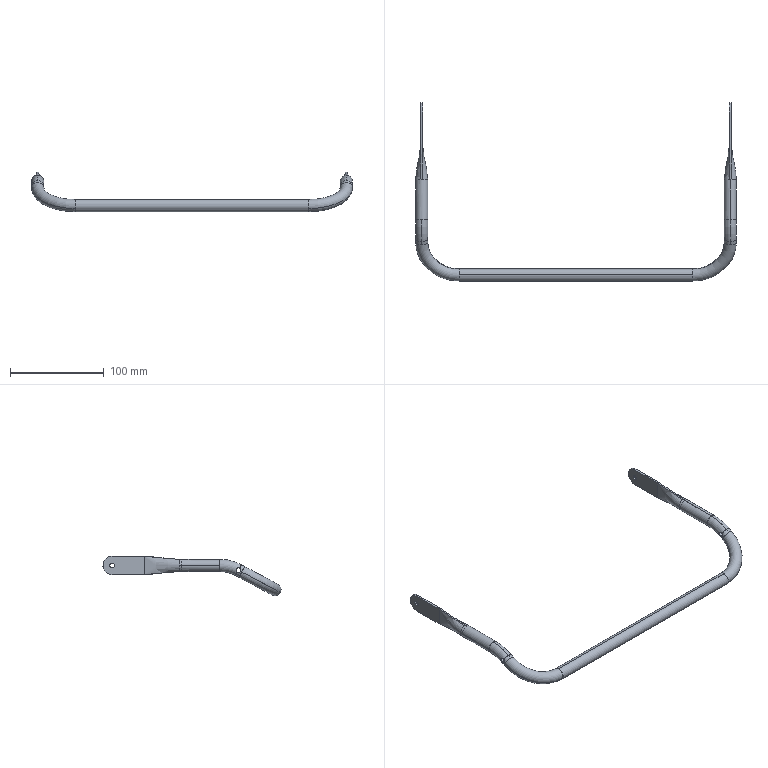Part | SolidWorks | features BaseBody 1 | 1 solid | 69 faces | box 342 x 189.784 x 41.985 mm | volume 25902 mm3 | cylinder 34 | torus 16 | plane 11 | spline 8 | commonest cylinder face diameters 5.2 x12 11.4 x10 13 x10 19.5 x2